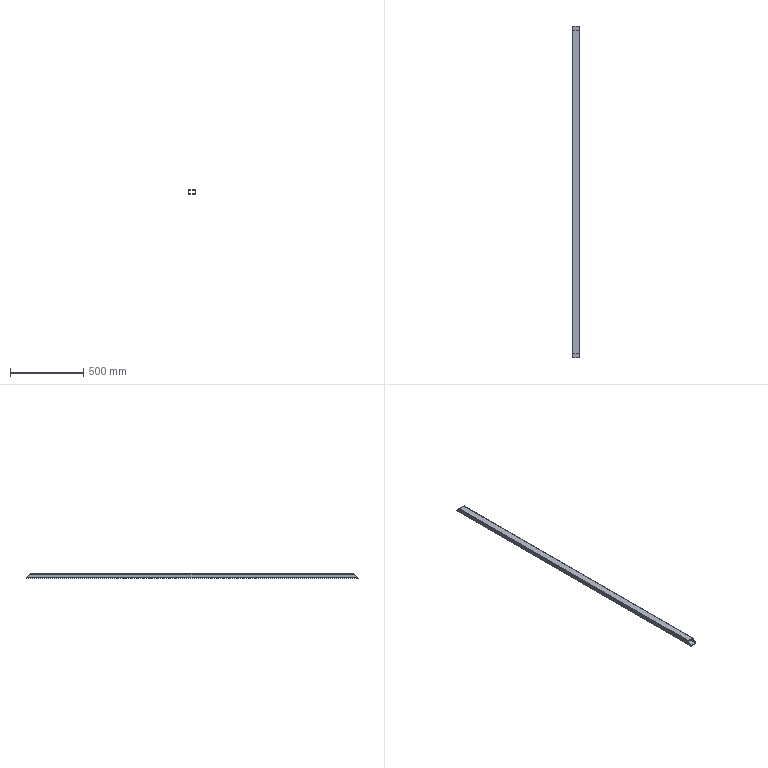Part | SolidWorks | features Extrusion 1, ICE 1 | 1 solid | 18 faces | box 50 x 2270 x 30 mm | volume 756578 mm3 | plane 10 | cylinder 8 | commonest cylinder face diameters 2.3 x4 6.9 x4
STEP:
#1=CARTESIAN_POINT('',(-22.7,2243.45,11.55));
#2=VERTEX_POINT('',#1);
#3=CARTESIAN_POINT('',(-22.7,2266.55,-11.55));
#4=VERTEX_POINT('',#3);
#5=CARTESIAN_POINT('',(-22.7,2256.725,-1.725));
#6=DIRECTION('',(0.,0.7071,-0.7071));
#7=VECTOR('',#6,1000.);
#8=LINE('',#5,#7);
#9=EDGE_CURVE('',#2,#4,#8,.T.);
#10=ORIENTED_EDGE('',*,*,#9,.F.);
#11=CARTESIAN_POINT('',(-22.7,26.55,11.55));
#12=VERTEX_POINT('',#11);
#13=CARTESIAN_POINT('',(-22.7,2270.,11.55));
#14=DIRECTION('',(0.,-1.,0.));
#15=VECTOR('',#14,1000.);
#16=LINE('',#13,#15);
#17=EDGE_CURVE('',#2,#12,#16,.T.);
#18=ORIENTED_EDGE('',*,*,#17,.T.);
#19=CARTESIAN_POINT('',(-22.7,3.45,-11.55));
#20=VERTEX_POINT('',#19);
#21=CARTESIAN_POINT('',(-22.7,1148.275,1133.275));
#22=DIRECTION('',(0.,0.7071,0.7071));
#23=VECTOR('',#22,1000.);
#24=LINE('',#21,#23);
#25=EDGE_CURVE('',#20,#12,#24,.T.);
#26=ORIENTED_EDGE('',*,*,#25,.F.);
#27=CARTESIAN_POINT('',(-22.7,2270.,-11.55));
#28=DIRECTION('',(0.,-1.,0.));
#29=VECTOR('',#28,1000.);
#30=LINE('',#27,#29);
#31=EDGE_CURVE('',#4,#20,#30,.T.);
#32=ORIENTED_EDGE('',*,*,#31,.F.);
#33=EDGE_LOOP('',(#10,#18,#26,#32));
#34=FACE_OUTER_BOUND('',#33,.T.);
#35=CARTESIAN_POINT('',(-22.7,2270.,11.55));
#36=DIRECTION('',(1.,0.,0.));
#37=DIRECTION('',(0.,0.,-1.));
#38=AXIS2_PLACEMENT_3D('',#35,#36,#37);
#39=PLANE('',#38);
#40=ADVANCED_FACE('',(#34),#39,.T.);
#41=CARTESIAN_POINT('',(-21.55,2267.7,-12.7));
#42=VERTEX_POINT('',#41);
#43=CARTESIAN_POINT('',(-22.7,2266.55,-11.55));
#44=CARTESIAN_POINT('',(-22.7,2267.224,-12.224));
#45=CARTESIAN_POINT('',(-22.224,2267.7,-12.7));
#46=CARTESIAN_POINT('',(-21.55,2267.7,-12.7));
#47=(BOUNDED_CURVE()B_SPLINE_CURVE(3,(#43,#44,#45,#46),.UNSPECIFIED.,.F.,.F.)B_SPLINE_CURVE_WITH_KNOTS((4,4),(1.571,3.142),.UNSPECIFIED.)CURVE()GEOMETRIC_REPRESENTATION_ITEM()RATIONAL_B_SPLINE_CURVE((1.,0.8047,0.8047,1.))REPRESENTATION_ITEM(''));
#48=EDGE_CURVE('',#4,#42,#47,.T.);
#49=ORIENTED_EDGE('',*,*,#48,.F.);
#50=ORIENTED_EDGE('',*,*,#31,.T.);
#51=CARTESIAN_POINT('',(-21.55,2.3,-12.7));
#52=VERTEX_POINT('',#51);
#53=CARTESIAN_POINT('',(-21.55,2.3,-12.7));
#54=CARTESIAN_POINT('',(-22.224,2.3,-12.7));
#55=CARTESIAN_POINT('',(-22.7,2.776,-12.224));
#56=CARTESIAN_POINT('',(-22.7,3.45,-11.55));
#57=(BOUNDED_CURVE()B_SPLINE_CURVE(3,(#53,#54,#55,#56),.UNSPECIFIED.,.F.,.F.)B_SPLINE_CURVE_WITH_KNOTS((4,4),(0.,1.571),.UNSPECIFIED.)CURVE()GEOMETRIC_REPRESENTATION_ITEM()RATIONAL_B_SPLINE_CURVE((1.,0.8047,0.8047,1.))REPRESENTATION_ITEM(''));
#58=EDGE_CURVE('',#52,#20,#57,.T.);
#59=ORIENTED_EDGE('',*,*,#58,.F.);
#60=CARTESIAN_POINT('',(-21.55,2270.,-12.7));
#61=DIRECTION('',(0.,-1.,0.));
#62=VECTOR('',#61,1000.);
#63=LINE('',#60,#62);
#64=EDGE_CURVE('',#42,#52,#63,.T.);
#65=ORIENTED_EDGE('',*,*,#64,.F.);
#66=EDGE_LOOP('',(#49,#50,#59,#65));
#67=FACE_OUTER_BOUND('',#66,.T.);
#68=CARTESIAN_POINT('',(-21.55,2270.,-11.55));
#69=DIRECTION('',(0.,-1.,0.));
#70=DIRECTION('',(0.,0.,-1.));
#71=AXIS2_PLACEMENT_3D('',#68,#69,#70);
#72=CYLINDRICAL_SURFACE('',#71,1.15);
#73=ADVANCED_FACE('',(#67),#72,.F.);
#74=CARTESIAN_POINT('',(21.55,2267.7,-12.7));
#75=VERTEX_POINT('',#74);
#76=CARTESIAN_POINT('',(-21.55,2267.7,-12.7));
#77=DIRECTION('',(1.,0.,0.));
#78=VECTOR('',#77,1000.);
#79=LINE('',#76,#78);
#80=EDGE_CURVE('',#42,#75,#79,.T.);
#81=ORIENTED_EDGE('',*,*,#80,.F.);
#82=ORIENTED_EDGE('',*,*,#64,.T.);
#83=CARTESIAN_POINT('',(21.55,2.3,-12.7));
#84=VERTEX_POINT('',#83);
#85=CARTESIAN_POINT('',(-21.55,2.3,-12.7));
#86=DIRECTION('',(-1.,0.,0.));
#87=VECTOR('',#86,1000.);
#88=LINE('',#85,#87);
#89=EDGE_CURVE('',#84,#52,#88,.T.);
#90=ORIENTED_EDGE('',*,*,#89,.F.);
#91=CARTESIAN_POINT('',(21.55,2270.,-12.7));
#92=DIRECTION('',(0.,-1.,0.));
#93=VECTOR('',#92,1000.);
#94=LINE('',#91,#93);
#95=EDGE_CURVE('',#75,#84,#94,.T.);
#96=ORIENTED_EDGE('',*,*,#95,.F.);
#97=EDGE_LOOP('',(#81,#82,#90,#96));
#98=FACE_OUTER_BOUND('',#97,.T.);
#99=CARTESIAN_POINT('',(-21.55,2270.,-12.7));
#100=DIRECTION('',(0.,0.,1.));
#101=DIRECTION('',(1.,0.,0.));
#102=AXIS2_PLACEMENT_3D('',#99,#100,#101);
#103=PLANE('',#102);
#104=ADVANCED_FACE('',(#98),#103,.T.);
#105=CARTESIAN_POINT('',(22.7,2266.55,-11.55));
#106=VERTEX_POINT('',#105);
#107=CARTESIAN_POINT('',(21.55,2267.7,-12.7));
#108=CARTESIAN_POINT('',(22.224,2267.7,-12.7));
#109=CARTESIAN_POINT('',(22.7,2267.224,-12.224));
#110=CARTESIAN_POINT('',(22.7,2266.55,-11.55));
#111=(BOUNDED_CURVE()B_SPLINE_CURVE(3,(#107,#108,#109,#110),.UNSPECIFIED.,.F.,.F.)B_SPLINE_CURVE_WITH_KNOTS((4,4),(3.142,4.712),.UNSPECIFIED.)CURVE()GEOMETRIC_REPRESENTATION_ITEM()RATIONAL_B_SPLINE_CURVE((1.,0.8047,0.8047,1.))REPRESENTATION_ITEM(''));
#112=EDGE_CURVE('',#75,#106,#111,.T.);
#113=ORIENTED_EDGE('',*,*,#112,.F.);
#114=ORIENTED_EDGE('',*,*,#95,.T.);
#115=CARTESIAN_POINT('',(22.7,3.45,-11.55));
#116=VERTEX_POINT('',#115);
#117=CARTESIAN_POINT('',(22.7,3.45,-11.55));
#118=CARTESIAN_POINT('',(22.7,2.776,-12.224));
#119=CARTESIAN_POINT('',(22.224,2.3,-12.7));
#120=CARTESIAN_POINT('',(21.55,2.3,-12.7));
#121=(BOUNDED_CURVE()B_SPLINE_CURVE(3,(#117,#118,#119,#120),.UNSPECIFIED.,.F.,.T.)B_SPLINE_CURVE_WITH_KNOTS((4,4),(4.712,6.283),.UNSPECIFIED.)CURVE()GEOMETRIC_REPRESENTATION_ITEM()RATIONAL_B_SPLINE_CURVE((1.,0.8047,0.8047,1.))REPRESENTATION_ITEM(''));
#122=EDGE_CURVE('',#116,#84,#121,.T.);
#123=ORIENTED_EDGE('',*,*,#122,.F.);
#124=CARTESIAN_POINT('',(22.7,2270.,-11.55));
#125=DIRECTION('',(0.,-1.,0.));
#126=VECTOR('',#125,1000.);
#127=LINE('',#124,#126);
#128=EDGE_CURVE('',#106,#116,#127,.T.);
#129=ORIENTED_EDGE('',*,*,#128,.F.);
#130=EDGE_LOOP('',(#113,#114,#123,#129));
#131=FACE_OUTER_BOUND('',#130,.T.);
#132=CARTESIAN_POINT('',(21.55,2270.,-11.55));
#133=DIRECTION('',(0.,-1.,0.));
#134=DIRECTION('',(0.,0.,-1.));
#135=AXIS2_PLACEMENT_3D('',#132,#133,#134);
#136=CYLINDRICAL_SURFACE('',#135,1.15);
#137=ADVANCED_FACE('',(#131),#136,.F.);
#138=CARTESIAN_POINT('',(22.7,2243.45,11.55));
#139=VERTEX_POINT('',#138);
#140=CARTESIAN_POINT('',(22.7,2256.725,-1.725));
#141=DIRECTION('',(0.,-0.7071,0.7071));
#142=VECTOR('',#141,1000.);
#143=LINE('',#140,#142);
#144=EDGE_CURVE('',#106,#139,#143,.T.);
#145=ORIENTED_EDGE('',*,*,#144,.F.);
#146=ORIENTED_EDGE('',*,*,#128,.T.);
#147=CARTESIAN_POINT('',(22.7,26.55,11.55));
#148=VERTEX_POINT('',#147);
#149=CARTESIAN_POINT('',(22.7,1148.275,1133.275));
#150=DIRECTION('',(0.,-0.7071,-0.7071));
#151=VECTOR('',#150,1000.);
#152=LINE('',#149,#151);
#153=EDGE_CURVE('',#148,#116,#152,.T.);
#154=ORIENTED_EDGE('',*,*,#153,.F.);
#155=CARTESIAN_POINT('',(22.7,2270.,11.55));
#156=DIRECTION('',(0.,-1.,0.));
#157=VECTOR('',#156,1000.);
#158=LINE('',#155,#157);
#159=EDGE_CURVE('',#139,#148,#158,.T.);
#160=ORIENTED_EDGE('',*,*,#159,.F.);
#161=EDGE_LOOP('',(#145,#146,#154,#160));
#162=FACE_OUTER_BOUND('',#161,.T.);
#163=CARTESIAN_POINT('',(22.7,2270.,11.55));
#164=DIRECTION('',(-1.,0.,0.));
#165=DIRECTION('',(0.,0.,1.));
#166=AXIS2_PLACEMENT_3D('',#163,#164,#165);
#167=PLANE('',#166);
#168=ADVANCED_FACE('',(#162),#167,.T.);
#169=CARTESIAN_POINT('',(21.55,2242.3,12.7));
#170=VERTEX_POINT('',#169);
#171=CARTESIAN_POINT('',(22.7,2243.45,11.55));
#172=CARTESIAN_POINT('',(22.7,2242.776,12.224));
#173=CARTESIAN_POINT('',(22.224,2242.3,12.7));
#174=CARTESIAN_POINT('',(21.55,2242.3,12.7));
#175=(BOUNDED_CURVE()B_SPLINE_CURVE(3,(#171,#172,#173,#174),.UNSPECIFIED.,.F.,.F.)B_SPLINE_CURVE_WITH_KNOTS((4,4),(4.712,6.283),.UNSPECIFIED.)CURVE()GEOMETRIC_REPRESENTATION_ITEM()RATIONAL_B_SPLINE_CURVE((1.,0.8047,0.8047,1.))REPRESENTATION_ITEM(''));
#176=EDGE_CURVE('',#139,#170,#175,.T.);
#177=ORIENTED_EDGE('',*,*,#176,.F.);
#178=ORIENTED_EDGE('',*,*,#159,.T.);
#179=CARTESIAN_POINT('',(21.55,27.7,12.7));
#180=VERTEX_POINT('',#179);
#181=CARTESIAN_POINT('',(21.55,27.7,12.7));
#182=CARTESIAN_POINT('',(22.224,27.7,12.7));
#183=CARTESIAN_POINT('',(22.7,27.224,12.224));
#184=CARTESIAN_POINT('',(22.7,26.55,11.55));
#185=(BOUNDED_CURVE()B_SPLINE_CURVE(3,(#181,#182,#183,#184),.UNSPECIFIED.,.F.,.F.)B_SPLINE_CURVE_WITH_KNOTS((4,4),(3.142,4.712),.UNSPECIFIED.)CURVE()GEOMETRIC_REPRESENTATION_ITEM()RATIONAL_B_SPLINE_CURVE((1.,0.8047,0.8047,1.))REPRESENTATION_ITEM(''));
#186=EDGE_CURVE('',#180,#148,#185,.T.);
#187=ORIENTED_EDGE('',*,*,#186,.F.);
#188=CARTESIAN_POINT('',(21.55,2270.,12.7));
#189=DIRECTION('',(0.,-1.,0.));
#190=VECTOR('',#189,1000.);
#191=LINE('',#188,#190);
#192=EDGE_CURVE('',#170,#180,#191,.T.);
#193=ORIENTED_EDGE('',*,*,#192,.F.);
#194=EDGE_LOOP('',(#177,#178,#187,#193));
#195=FACE_OUTER_BOUND('',#194,.T.);
#196=CARTESIAN_POINT('',(21.55,2270.,11.55));
#197=DIRECTION('',(0.,-1.,0.));
#198=DIRECTION('',(0.,0.,-1.));
#199=AXIS2_PLACEMENT_3D('',#196,#197,#198);
#200=CYLINDRICAL_SURFACE('',#199,1.15);
#201=ADVANCED_FACE('',(#195),#200,.F.);
#202=CARTESIAN_POINT('',(-21.55,2242.3,12.7));
#203=VERTEX_POINT('',#202);
#204=CARTESIAN_POINT('',(-21.55,2242.3,12.7));
#205=DIRECTION('',(-1.,0.,0.));
#206=VECTOR('',#205,1000.);
#207=LINE('',#204,#206);
#208=EDGE_CURVE('',#170,#203,#207,.T.);
#209=ORIENTED_EDGE('',*,*,#208,.F.);
#210=ORIENTED_EDGE('',*,*,#192,.T.);
#211=CARTESIAN_POINT('',(-21.55,27.7,12.7));
#212=VERTEX_POINT('',#211);
#213=CARTESIAN_POINT('',(-21.55,27.7,12.7));
#214=DIRECTION('',(1.,0.,0.));
#215=VECTOR('',#214,1000.);
#216=LINE('',#213,#215);
#217=EDGE_CURVE('',#212,#180,#216,.T.);
#218=ORIENTED_EDGE('',*,*,#217,.F.);
#219=CARTESIAN_POINT('',(-21.55,2270.,12.7));
#220=DIRECTION('',(0.,-1.,0.));
#221=VECTOR('',#220,1000.);
#222=LINE('',#219,#221);
#223=EDGE_CURVE('',#203,#212,#222,.T.);
#224=ORIENTED_EDGE('',*,*,#223,.F.);
#225=EDGE_LOOP('',(#209,#210,#218,#224));
#226=FACE_OUTER_BOUND('',#225,.T.);
#227=CARTESIAN_POINT('',(-21.55,2270.,12.7));
#228=DIRECTION('',(0.,0.,-1.));
#229=DIRECTION('',(-1.,0.,0.));
#230=AXIS2_PLACEMENT_3D('',#227,#228,#229);
#231=PLANE('',#230);
#232=ADVANCED_FACE('',(#226),#231,.T.);
#233=CARTESIAN_POINT('',(-21.55,2242.3,12.7));
#234=CARTESIAN_POINT('',(-22.224,2242.3,12.7));
#235=CARTESIAN_POINT('',(-22.7,2242.776,12.224));
#236=CARTESIAN_POINT('',(-22.7,2243.45,11.55));
#237=(BOUNDED_CURVE()B_SPLINE_CURVE(3,(#233,#234,#235,#236),.UNSPECIFIED.,.F.,.F.)B_SPLINE_CURVE_WITH_KNOTS((4,4),(0.,1.571),.UNSPECIFIED.)CURVE()GEOMETRIC_REPRESENTATION_ITEM()RATIONAL_B_SPLINE_CURVE((1.,0.8047,0.8047,1.))REPRESENTATION_ITEM(''));
#238=EDGE_CURVE('',#203,#2,#237,.T.);
#239=ORIENTED_EDGE('',*,*,#238,.F.);
#240=ORIENTED_EDGE('',*,*,#223,.T.);
#241=CARTESIAN_POINT('',(-22.7,26.55,11.55));
#242=CARTESIAN_POINT('',(-22.7,27.224,12.224));
#243=CARTESIAN_POINT('',(-22.224,27.7,12.7));
#244=CARTESIAN_POINT('',(-21.55,27.7,12.7));
#245=(BOUNDED_CURVE()B_SPLINE_CURVE(3,(#241,#242,#243,#244),.UNSPECIFIED.,.F.,.T.)B_SPLINE_CURVE_WITH_KNOTS((4,4),(1.571,3.142),.UNSPECIFIED.)CURVE()GEOMETRIC_REPRESENTATION_ITEM()RATIONAL_B_SPLINE_CURVE((1.,0.8047,0.8047,1.))REPRESENTATION_ITEM(''));
#246=EDGE_CURVE('',#12,#212,#245,.T.);
#247=ORIENTED_EDGE('',*,*,#246,.F.);
#248=ORIENTED_EDGE('',*,*,#17,.F.);
#249=EDGE_LOOP('',(#239,#240,#247,#248));
#250=FACE_OUTER_BOUND('',#249,.T.);
#251=CARTESIAN_POINT('',(-21.55,2270.,11.55));
#252=DIRECTION('',(0.,-1.,0.));
#253=DIRECTION('',(0.,0.,-1.));
#254=AXIS2_PLACEMENT_3D('',#251,#252,#253);
#255=CYLINDRICAL_SURFACE('',#254,1.15);
#256=ADVANCED_FACE('',(#250),#255,.F.);
#257=ORIENTED_EDGE('',*,*,#246,.T.);
#258=ORIENTED_EDGE('',*,*,#217,.T.);
#259=ORIENTED_EDGE('',*,*,#186,.T.);
#260=ORIENTED_EDGE('',*,*,#153,.T.);
#261=ORIENTED_EDGE('',*,*,#122,.T.);
#262=ORIENTED_EDGE('',*,*,#89,.T.);
#263=ORIENTED_EDGE('',*,*,#58,.T.);
#264=ORIENTED_EDGE('',*,*,#25,.T.);
#265=EDGE_LOOP('',(#257,#258,#259,#260,#261,#262,#263,#264));
#266=FACE_BOUND('',#265,.T.);
#267=CARTESIAN_POINT('',(21.55,0.,-15.));
#268=VERTEX_POINT('',#267);
#269=CARTESIAN_POINT('',(-21.55,0.,-15.));
#270=VERTEX_POINT('',#269);
#271=CARTESIAN_POINT('',(-21.55,0.,-15.));
#272=DIRECTION('',(-1.,0.,0.));
#273=VECTOR('',#272,1000.);
#274=LINE('',#271,#273);
#275=EDGE_CURVE('',#268,#270,#274,.T.);
#276=ORIENTED_EDGE('',*,*,#275,.F.);
#277=CARTESIAN_POINT('',(25.,3.45,-11.55));
#278=VERTEX_POINT('',#277);
#279=CARTESIAN_POINT('',(25.,3.45,-11.55));
#280=CARTESIAN_POINT('',(25.,1.429,-13.571));
#281=CARTESIAN_POINT('',(23.571,0.,-15.));
#282=CARTESIAN_POINT('',(21.55,0.,-15.));
#283=(BOUNDED_CURVE()B_SPLINE_CURVE(3,(#279,#280,#281,#282),.UNSPECIFIED.,.F.,.T.)B_SPLINE_CURVE_WITH_KNOTS((4,4),(4.712,6.283),.UNSPECIFIED.)CURVE()GEOMETRIC_REPRESENTATION_ITEM()RATIONAL_B_SPLINE_CURVE((1.,0.8047,0.8047,1.))REPRESENTATION_ITEM(''));
#284=EDGE_CURVE('',#278,#268,#283,.T.);
#285=ORIENTED_EDGE('',*,*,#284,.F.);
#286=CARTESIAN_POINT('',(25.,26.55,11.55));
#287=VERTEX_POINT('',#286);
#288=CARTESIAN_POINT('',(25.,1148.275,1133.275));
#289=DIRECTION('',(0.,-0.7071,-0.7071));
#290=VECTOR('',#289,1000.);
#291=LINE('',#288,#290);
#292=EDGE_CURVE('',#287,#278,#291,.T.);
#293=ORIENTED_EDGE('',*,*,#292,.F.);
#294=CARTESIAN_POINT('',(21.55,30.,15.));
#295=VERTEX_POINT('',#294);
#296=CARTESIAN_POINT('',(21.55,30.,15.));
#297=CARTESIAN_POINT('',(23.571,30.,15.));
#298=CARTESIAN_POINT('',(25.,28.571,13.571));
#299=CARTESIAN_POINT('',(25.,26.55,11.55));
#300=(BOUNDED_CURVE()B_SPLINE_CURVE(3,(#296,#297,#298,#299),.UNSPECIFIED.,.F.,.F.)B_SPLINE_CURVE_WITH_KNOTS((4,4),(3.142,4.712),.UNSPECIFIED.)CURVE()GEOMETRIC_REPRESENTATION_ITEM()RATIONAL_B_SPLINE_CURVE((1.,0.8047,0.8047,1.))REPRESENTATION_ITEM(''));
#301=EDGE_CURVE('',#295,#287,#300,.T.);
#302=ORIENTED_EDGE('',*,*,#301,.F.);
#303=CARTESIAN_POINT('',(-21.55,30.,15.));
#304=VERTEX_POINT('',#303);
#305=CARTESIAN_POINT('',(-25.,30.,15.));
#306=DIRECTION('',(1.,0.,0.));
#307=VECTOR('',#306,1000.);
#308=LINE('',#305,#307);
#309=EDGE_CURVE('',#304,#295,#308,.T.);
#310=ORIENTED_EDGE('',*,*,#309,.F.);
#311=CARTESIAN_POINT('',(-25.,26.55,11.55));
#312=VERTEX_POINT('',#311);
#313=CARTESIAN_POINT('',(-25.,26.55,11.55));
#314=CARTESIAN_POINT('',(-25.,28.571,13.571));
#315=CARTESIAN_POINT('',(-23.571,30.,15.));
#316=CARTESIAN_POINT('',(-21.55,30.,15.));
#317=(BOUNDED_CURVE()B_SPLINE_CURVE(3,(#313,#314,#315,#316),.UNSPECIFIED.,.F.,.F.)B_SPLINE_CURVE_WITH_KNOTS((4,4),(1.571,3.142),.UNSPECIFIED.)CURVE()GEOMETRIC_REPRESENTATION_ITEM()RATIONAL_B_SPLINE_CURVE((1.,0.8047,0.8047,1.))REPRESENTATION_ITEM(''));
#318=EDGE_CURVE('',#312,#304,#317,.T.);
#319=ORIENTED_EDGE('',*,*,#318,.F.);
#320=CARTESIAN_POINT('',(-25.,3.45,-11.55));
#321=VERTEX_POINT('',#320);
#322=CARTESIAN_POINT('',(-25.,30.,15.));
#323=DIRECTION('',(0.,0.7071,0.7071));
#324=VECTOR('',#323,1000.);
#325=LINE('',#322,#324);
#326=EDGE_CURVE('',#321,#312,#325,.T.);
#327=ORIENTED_EDGE('',*,*,#326,.F.);
#328=CARTESIAN_POINT('',(-21.55,0.,-15.));
#329=CARTESIAN_POINT('',(-23.571,0.,-15.));
#330=CARTESIAN_POINT('',(-25.,1.429,-13.571));
#331=CARTESIAN_POINT('',(-25.,3.45,-11.55));
#332=(BOUNDED_CURVE()B_SPLINE_CURVE(3,(#328,#329,#330,#331),.UNSPECIFIED.,.F.,.T.)B_SPLINE_CURVE_WITH_KNOTS((4,4),(0.,1.571),.UNSPECIFIED.)CURVE()GEOMETRIC_REPRESENTATION_ITEM()RATIONAL_B_SPLINE_CURVE((1.,0.8047,0.8047,1.))REPRESENTATION_ITEM(''));
#333=EDGE_CURVE('',#270,#321,#332,.T.);
#334=ORIENTED_EDGE('',*,*,#333,.F.);
#335=EDGE_LOOP('',(#276,#285,#293,#302,#310,#319,#327,#334));
#336=FACE_OUTER_BOUND('',#335,.T.);
#337=CARTESIAN_POINT('',(-25.,30.,15.));
#338=DIRECTION('',(0.,0.7071,-0.7071));
#339=DIRECTION('',(0.,0.7071,0.7071));
#340=AXIS2_PLACEMENT_3D('',#337,#338,#339);
#341=PLANE('',#340);
#342=ADVANCED_FACE('',(#266,#336),#341,.F.);
#343=ORIENTED_EDGE('',*,*,#238,.T.);
#344=ORIENTED_EDGE('',*,*,#9,.T.);
#345=ORIENTED_EDGE('',*,*,#48,.T.);
#346=ORIENTED_EDGE('',*,*,#80,.T.);
#347=ORIENTED_EDGE('',*,*,#112,.T.);
#348=ORIENTED_EDGE('',*,*,#144,.T.);
#349=ORIENTED_EDGE('',*,*,#176,.T.);
#350=ORIENTED_EDGE('',*,*,#208,.T.);
#351=EDGE_LOOP('',(#343,#344,#345,#346,#347,#348,#349,#350));
#352=FACE_BOUND('',#351,.T.);
#353=CARTESIAN_POINT('',(-25.,2243.45,11.55));
#354=VERTEX_POINT('',#353);
#355=CARTESIAN_POINT('',(-25.,2266.55,-11.55));
#356=VERTEX_POINT('',#355);
#357=CARTESIAN_POINT('',(-25.,2270.,-15.));
#358=DIRECTION('',(0.,0.7071,-0.7071));
#359=VECTOR('',#358,1000.);
#360=LINE('',#357,#359);
#361=EDGE_CURVE('',#354,#356,#360,.T.);
#362=ORIENTED_EDGE('',*,*,#361,.F.);
#363=CARTESIAN_POINT('',(-21.55,2240.,15.));
#364=VERTEX_POINT('',#363);
#365=CARTESIAN_POINT('',(-21.55,2240.,15.));
#366=CARTESIAN_POINT('',(-23.571,2240.,15.));
#367=CARTESIAN_POINT('',(-25.,2241.429,13.571));
#368=CARTESIAN_POINT('',(-25.,2243.45,11.55));
#369=(BOUNDED_CURVE()B_SPLINE_CURVE(3,(#365,#366,#367,#368),.UNSPECIFIED.,.F.,.F.)B_SPLINE_CURVE_WITH_KNOTS((4,4),(0.,1.571),.UNSPECIFIED.)CURVE()GEOMETRIC_REPRESENTATION_ITEM()RATIONAL_B_SPLINE_CURVE((1.,0.8047,0.8047,1.))REPRESENTATION_ITEM(''));
#370=EDGE_CURVE('',#364,#354,#369,.T.);
#371=ORIENTED_EDGE('',*,*,#370,.F.);
#372=CARTESIAN_POINT('',(21.55,2240.,15.));
#373=VERTEX_POINT('',#372);
#374=CARTESIAN_POINT('',(-25.,2240.,15.));
#375=DIRECTION('',(1.,0.,0.));
#376=VECTOR('',#375,1000.);
#377=LINE('',#374,#376);
#378=EDGE_CURVE('',#364,#373,#377,.T.);
#379=ORIENTED_EDGE('',*,*,#378,.T.);
#380=CARTESIAN_POINT('',(25.,2243.45,11.55));
#381=VERTEX_POINT('',#380);
#382=CARTESIAN_POINT('',(25.,2243.45,11.55));
#383=CARTESIAN_POINT('',(25.,2241.429,13.571));
#384=CARTESIAN_POINT('',(23.571,2240.,15.));
#385=CARTESIAN_POINT('',(21.55,2240.,15.));
#386=(BOUNDED_CURVE()B_SPLINE_CURVE(3,(#382,#383,#384,#385),.UNSPECIFIED.,.F.,.F.)B_SPLINE_CURVE_WITH_KNOTS((4,4),(4.712,6.283),.UNSPECIFIED.)CURVE()GEOMETRIC_REPRESENTATION_ITEM()RATIONAL_B_SPLINE_CURVE((1.,0.8047,0.8047,1.))REPRESENTATION_ITEM(''));
#387=EDGE_CURVE('',#381,#373,#386,.T.);
#388=ORIENTED_EDGE('',*,*,#387,.F.);
#389=CARTESIAN_POINT('',(25.,2266.55,-11.55));
#390=VERTEX_POINT('',#389);
#391=CARTESIAN_POINT('',(25.,2256.725,-1.725));
#392=DIRECTION('',(0.,-0.7071,0.7071));
#393=VECTOR('',#392,1000.);
#394=LINE('',#391,#393);
#395=EDGE_CURVE('',#390,#381,#394,.T.);
#396=ORIENTED_EDGE('',*,*,#395,.F.);
#397=CARTESIAN_POINT('',(21.55,2270.,-15.));
#398=VERTEX_POINT('',#397);
#399=CARTESIAN_POINT('',(21.55,2270.,-15.));
#400=CARTESIAN_POINT('',(23.571,2270.,-15.));
#401=CARTESIAN_POINT('',(25.,2268.571,-13.571));
#402=CARTESIAN_POINT('',(25.,2266.55,-11.55));
#403=(BOUNDED_CURVE()B_SPLINE_CURVE(3,(#399,#400,#401,#402),.UNSPECIFIED.,.F.,.F.)B_SPLINE_CURVE_WITH_KNOTS((4,4),(3.142,4.712),.UNSPECIFIED.)CURVE()GEOMETRIC_REPRESENTATION_ITEM()RATIONAL_B_SPLINE_CURVE((1.,0.8047,0.8047,1.))REPRESENTATION_ITEM(''));
#404=EDGE_CURVE('',#398,#390,#403,.T.);
#405=ORIENTED_EDGE('',*,*,#404,.F.);
#406=CARTESIAN_POINT('',(-21.55,2270.,-15.));
#407=VERTEX_POINT('',#406);
#408=CARTESIAN_POINT('',(-21.55,2270.,-15.));
#409=DIRECTION('',(-1.,0.,0.));
#410=VECTOR('',#409,1000.);
#411=LINE('',#408,#410);
#412=EDGE_CURVE('',#398,#407,#411,.T.);
#413=ORIENTED_EDGE('',*,*,#412,.T.);
#414=CARTESIAN_POINT('',(-25.,2266.55,-11.55));
#415=CARTESIAN_POINT('',(-25.,2268.571,-13.571));
#416=CARTESIAN_POINT('',(-23.571,2270.,-15.));
#417=CARTESIAN_POINT('',(-21.55,2270.,-15.));
#418=(BOUNDED_CURVE()B_SPLINE_CURVE(3,(#414,#415,#416,#417),.UNSPECIFIED.,.F.,.F.)B_SPLINE_CURVE_WITH_KNOTS((4,4),(1.571,3.142),.UNSPECIFIED.)CURVE()GEOMETRIC_REPRESENTATION_ITEM()RATIONAL_B_SPLINE_CURVE((1.,0.8047,0.8047,1.))REPRESENTATION_ITEM(''));
#419=EDGE_CURVE('',#356,#407,#418,.T.);
#420=ORIENTED_EDGE('',*,*,#419,.F.);
#421=EDGE_LOOP('',(#362,#371,#379,#388,#396,#405,#413,#420));
#422=FACE_OUTER_BOUND('',#421,.T.);
#423=CARTESIAN_POINT('',(-25.,2270.,-15.));
#424=DIRECTION('',(0.,-0.7071,-0.7071));
#425=DIRECTION('',(0.,0.7071,-0.7071));
#426=AXIS2_PLACEMENT_3D('',#423,#424,#425);
#427=PLANE('',#426);
#428=ADVANCED_FACE('',(#352,#422),#427,.F.);
#429=CARTESIAN_POINT('',(21.55,2270.,-15.));
#430=DIRECTION('',(0.,-1.,0.));
#431=VECTOR('',#430,1000.);
#432=LINE('',#429,#431);
#433=EDGE_CURVE('',#398,#268,#432,.T.);
#434=ORIENTED_EDGE('',*,*,#433,.F.);
#435=ORIENTED_EDGE('',*,*,#404,.T.);
#436=CARTESIAN_POINT('',(25.,2270.,-11.55));
#437=DIRECTION('',(0.,-1.,0.));
#438=VECTOR('',#437,1000.);
#439=LINE('',#436,#438);
#440=EDGE_CURVE('',#390,#278,#439,.T.);
#441=ORIENTED_EDGE('',*,*,#440,.T.);
#442=ORIENTED_EDGE('',*,*,#284,.T.);
#443=EDGE_LOOP('',(#434,#435,#441,#442));
#444=FACE_OUTER_BOUND('',#443,.T.);
#445=CARTESIAN_POINT('',(21.55,2270.,-11.55));
#446=DIRECTION('',(0.,-1.,0.));
#447=DIRECTION('',(0.,0.,-1.));
#448=AXIS2_PLACEMENT_3D('',#445,#446,#447);
#449=CYLINDRICAL_SURFACE('',#448,3.45);
#450=ADVANCED_FACE('',(#444),#449,.T.);
#451=ORIENTED_EDGE('',*,*,#275,.T.);
#452=CARTESIAN_POINT('',(-21.55,2270.,-15.));
#453=DIRECTION('',(0.,-1.,0.));
#454=VECTOR('',#453,1000.);
#455=LINE('',#452,#454);
#456=EDGE_CURVE('',#407,#270,#455,.T.);
#457=ORIENTED_EDGE('',*,*,#456,.F.);
#458=ORIENTED_EDGE('',*,*,#412,.F.);
#459=ORIENTED_EDGE('',*,*,#433,.T.);
#460=EDGE_LOOP('',(#451,#457,#458,#459));
#461=FACE_OUTER_BOUND('',#460,.T.);
#462=CARTESIAN_POINT('',(-21.55,2270.,-15.));
#463=DIRECTION('',(0.,0.,1.));
#464=DIRECTION('',(1.,0.,0.));
#465=AXIS2_PLACEMENT_3D('',#462,#463,#464);
#466=PLANE('',#465);
#467=ADVANCED_FACE('',(#461),#466,.F.);
#468=CARTESIAN_POINT('',(-25.,2270.,-11.55));
#469=DIRECTION('',(0.,-1.,0.));
#470=VECTOR('',#469,1000.);
#471=LINE('',#468,#470);
#472=EDGE_CURVE('',#356,#321,#471,.T.);
#473=ORIENTED_EDGE('',*,*,#472,.F.);
#474=ORIENTED_EDGE('',*,*,#419,.T.);
#475=ORIENTED_EDGE('',*,*,#456,.T.);
#476=ORIENTED_EDGE('',*,*,#333,.T.);
#477=EDGE_LOOP('',(#473,#474,#475,#476));
#478=FACE_OUTER_BOUND('',#477,.T.);
#479=CARTESIAN_POINT('',(-21.55,2270.,-11.55));
#480=DIRECTION('',(0.,-1.,0.));
#481=DIRECTION('',(0.,0.,-1.));
#482=AXIS2_PLACEMENT_3D('',#479,#480,#481);
#483=CYLINDRICAL_SURFACE('',#482,3.45);
#484=ADVANCED_FACE('',(#478),#483,.T.);
#485=CARTESIAN_POINT('',(-25.,2270.,11.55));
#486=DIRECTION('',(0.,-1.,0.));
#487=VECTOR('',#486,1000.);
#488=LINE('',#485,#487);
#489=EDGE_CURVE('',#354,#312,#488,.T.);
#490=ORIENTED_EDGE('',*,*,#489,.F.);
#491=ORIENTED_EDGE('',*,*,#361,.T.);
#492=ORIENTED_EDGE('',*,*,#472,.T.);
#493=ORIENTED_EDGE('',*,*,#326,.T.);
#494=EDGE_LOOP('',(#490,#491,#492,#493));
#495=FACE_OUTER_BOUND('',#494,.T.);
#496=CARTESIAN_POINT('',(-25.,2270.,11.55));
#497=DIRECTION('',(1.,0.,0.));
#498=DIRECTION('',(0.,0.,-1.));
#499=AXIS2_PLACEMENT_3D('',#496,#497,#498);
#500=PLANE('',#499);
#501=ADVANCED_FACE('',(#495),#500,.F.);
#502=CARTESIAN_POINT('',(-21.55,2270.,15.));
#503=DIRECTION('',(0.,-1.,0.));
#504=VECTOR('',#503,1000.);
#505=LINE('',#502,#504);
#506=EDGE_CURVE('',#364,#304,#505,.T.);
#507=ORIENTED_EDGE('',*,*,#506,.F.);
#508=ORIENTED_EDGE('',*,*,#370,.T.);
#509=ORIENTED_EDGE('',*,*,#489,.T.);
#510=ORIENTED_EDGE('',*,*,#318,.T.);
#511=EDGE_LOOP('',(#507,#508,#509,#510));
#512=FACE_OUTER_BOUND('',#511,.T.);
#513=CARTESIAN_POINT('',(-21.55,2270.,11.55));
#514=DIRECTION('',(0.,-1.,0.));
#515=DIRECTION('',(0.,0.,-1.));
#516=AXIS2_PLACEMENT_3D('',#513,#514,#515);
#517=CYLINDRICAL_SURFACE('',#516,3.45);
#518=ADVANCED_FACE('',(#512),#517,.T.);
#519=CARTESIAN_POINT('',(21.55,2270.,15.));
#520=DIRECTION('',(0.,-1.,0.));
#521=VECTOR('',#520,1000.);
#522=LINE('',#519,#521);
#523=EDGE_CURVE('',#373,#295,#522,.T.);
#524=ORIENTED_EDGE('',*,*,#523,.F.);
#525=ORIENTED_EDGE('',*,*,#378,.F.);
#526=ORIENTED_EDGE('',*,*,#506,.T.);
#527=ORIENTED_EDGE('',*,*,#309,.T.);
#528=EDGE_LOOP('',(#524,#525,#526,#527));
#529=FACE_OUTER_BOUND('',#528,.T.);
#530=CARTESIAN_POINT('',(-21.55,2270.,15.));
#531=DIRECTION('',(0.,0.,-1.));
#532=DIRECTION('',(-1.,0.,0.));
#533=AXIS2_PLACEMENT_3D('',#530,#531,#532);
#534=PLANE('',#533);
#535=ADVANCED_FACE('',(#529),#534,.F.);
#536=CARTESIAN_POINT('',(25.,2270.,11.55));
#537=DIRECTION('',(0.,-1.,0.));
#538=VECTOR('',#537,1000.);
#539=LINE('',#536,#538);
#540=EDGE_CURVE('',#381,#287,#539,.T.);
#541=ORIENTED_EDGE('',*,*,#540,.F.);
#542=ORIENTED_EDGE('',*,*,#387,.T.);
#543=ORIENTED_EDGE('',*,*,#523,.T.);
#544=ORIENTED_EDGE('',*,*,#301,.T.);
#545=EDGE_LOOP('',(#541,#542,#543,#544));
#546=FACE_OUTER_BOUND('',#545,.T.);
#547=CARTESIAN_POINT('',(21.55,2270.,11.55));
#548=DIRECTION('',(0.,-1.,0.));
#549=DIRECTION('',(0.,0.,-1.));
#550=AXIS2_PLACEMENT_3D('',#547,#548,#549);
#551=CYLINDRICAL_SURFACE('',#550,3.45);
#552=ADVANCED_FACE('',(#546),#551,.T.);
#553=ORIENTED_EDGE('',*,*,#440,.F.);
#554=ORIENTED_EDGE('',*,*,#395,.T.);
#555=ORIENTED_EDGE('',*,*,#540,.T.);
#556=ORIENTED_EDGE('',*,*,#292,.T.);
#557=EDGE_LOOP('',(#553,#554,#555,#556));
#558=FACE_OUTER_BOUND('',#557,.T.);
#559=CARTESIAN_POINT('',(25.,2270.,11.55));
#560=DIRECTION('',(-1.,0.,0.));
#561=DIRECTION('',(0.,0.,1.));
#562=AXIS2_PLACEMENT_3D('',#559,#560,#561);
#563=PLANE('',#562);
#564=ADVANCED_FACE('',(#558),#563,.F.);
#565=CLOSED_SHELL('',(#40,#73,#104,#137,#168,#201,#232,#256,#342,#428,#450,#467,#484,#501,#518,#535,#552,#564));
#566=MANIFOLD_SOLID_BREP('',#565);
#567=CARTESIAN_POINT('',(0.,0.,0.));
#568=DIRECTION('',(0.,0.,1.));
#569=DIRECTION('',(1.,0.,0.));
#570=AXIS2_PLACEMENT_3D('',#567,#568,#569);
#571=(LENGTH_UNIT()NAMED_UNIT(*)SI_UNIT(.MILLI.,.METRE.));
#572=UNCERTAINTY_MEASURE_WITH_UNIT(LENGTH_MEASURE(0.00001),#571,'','');
#573=(NAMED_UNIT(*)PLANE_ANGLE_UNIT()SI_UNIT($,.RADIAN.));
#574=(NAMED_UNIT(*)SI_UNIT($,.STERADIAN.)SOLID_ANGLE_UNIT());
#575=(GEOMETRIC_REPRESENTATION_CONTEXT(3)GLOBAL_UNCERTAINTY_ASSIGNED_CONTEXT((#572))GLOBAL_UNIT_ASSIGNED_CONTEXT((#571,#573,#574))REPRESENTATION_CONTEXT('',''));
#576=ADVANCED_BREP_SHAPE_REPRESENTATION('',(#566,#570),#575);